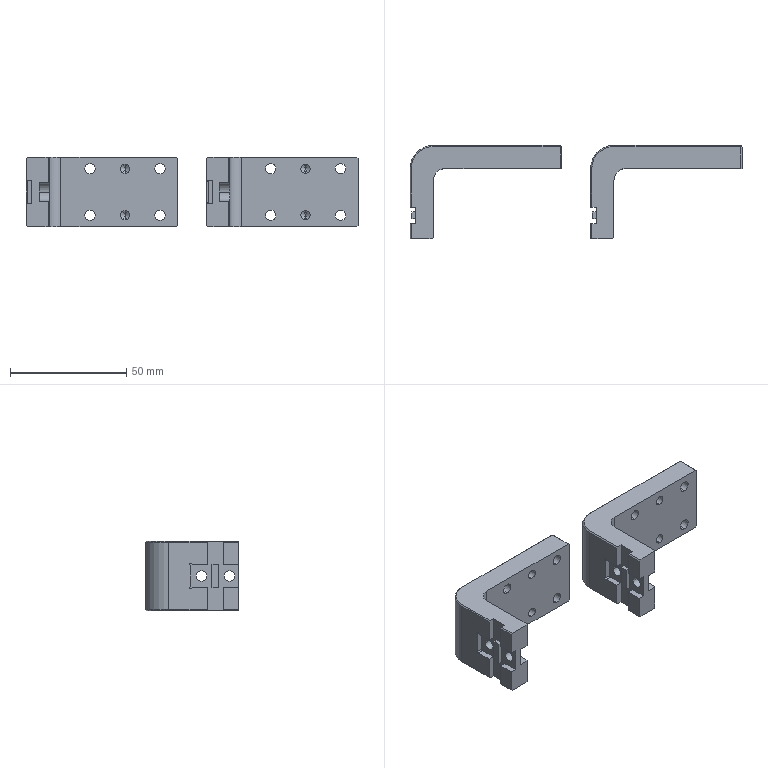NC program | NX | posted with a generic post | part box 142.5 x 40 x 30 mm
Whole program:
N10 G17 G21 G94 G90
(HOLE_MILLING , TOOL : D6)
N12 T12 M6
N14 G54
N16 G17 G0 G90 X-63.75 Y-5. B0. C0. S9500 M3
N18 G43 Z30. H12
N20 Z0.5
N22 G94 G3 X-64.25 Y-4.5 R0.5 F1500.
N24 X-64.75 Y-5. R0.5
N26 X-64.75 Y-5. Z0. I1. J0.
N28 X-64.75 Y-5. Z-0.5 I1. J0.
N30 X-64.75 Y-5. Z-1. I1. J0.
N32 X-64.75 Y-5. Z-1.5 I1. J0.
N34 X-64.75 Y-5. Z-2. I1. J0.
N36 X-64.75 Y-5. Z-2.5 I1. J0.
N38 X-64.75 Y-5. Z-3. I1. J0.
N40 X-64.75 Y-5. Z-3.5 I1. J0.
N42 X-64.75 Y-5. Z-4. I1. J0.
N44 X-64.75 Y-5. Z-4.5 I1. J0.
N46 X-64.059 Y-5.951 Z-4.6 R1.
N48 X-62.799 Y-5.309 R1.
N50 X-64.059 Y-5.951 R-1.
N52 X-63.429 Y-5.63 R0.5
N54 X-63.75 Y-5. R0.5
N56 G0 Z30.
N58 Y-25.
N60 Z0.5
N62 G3 X-64.25 Y-24.5 R0.5
N64 X-64.75 Y-25. R0.5
N66 X-64.75 Y-25. Z0. I1. J0.
N68 X-64.75 Y-25. Z-0.5 I1. J0.
N70 X-64.75 Y-25. Z-1. I1. J0.
N72 X-64.75 Y-25. Z-1.5 I1. J0.
N74 X-64.75 Y-25. Z-2. I1. J0.
N76 X-64.75 Y-25. Z-2.5 I1. J0.
N78 X-64.75 Y-25. Z-3. I1. J0.
N80 X-64.75 Y-25. Z-3.5 I1. J0.
N82 X-64.75 Y-25. Z-4. I1. J0.
N84 X-64.75 Y-25. Z-4.5 I1. J0.
N86 X-64.059 Y-25.951 Z-4.6 R1.
N88 X-62.799 Y-25.309 R1.
N90 X-64.059 Y-25.951 R-1.
N92 X-63.429 Y-25.63 R0.5
N94 X-63.75 Y-25. R0.5
N96 G0 Z30.
N98 X-33.75
N100 Z0.5
N102 G3 X-34.25 Y-24.5 R0.5
N104 X-34.75 Y-25. R0.5
N106 X-34.75 Y-25. Z0. I1. J0.
N108 X-34.75 Y-25. Z-0.5 I1. J0.
N110 X-34.75 Y-25. Z-1. I1. J0.
N112 X-34.75 Y-25. Z-1.5 I1. J0.
N114 X-34.75 Y-25. Z-2. I1. J0.
N116 X-34.75 Y-25. Z-2.5 I1. J0.
N118 X-34.75 Y-25. Z-3. I1. J0.
N120 X-34.75 Y-25. Z-3.5 I1. J0.
N122 X-34.75 Y-25. Z-4. I1. J0.
N124 X-34.75 Y-25. Z-4.5 I1. J0.
N126 X-34.059 Y-25.951 Z-4.6 R1.
N128 X-32.799 Y-25.309 R1.
N130 X-34.059 Y-25.951 R-1.
N132 X-33.429 Y-25.63 R0.5
N134 X-33.75 Y-25. R0.5
N136 G0 Z30.
N138 Y-5.
N140 Z0.5
N142 G3 X-34.25 Y-4.5 R0.5
N144 X-34.75 Y-5. R0.5
N146 X-34.75 Y-5. Z0. I1. J0.
N148 X-34.75 Y-5. Z-0.5 I1. J0.
N150 X-34.75 Y-5. Z-1. I1. J0.
N152 X-34.75 Y-5. Z-1.5 I1. J0.
N154 X-34.75 Y-5. Z-2. I1. J0.
N156 X-34.75 Y-5. Z-2.5 I1. J0.
N158 X-34.75 Y-5. Z-3. I1. J0.
N160 X-34.75 Y-5. Z-3.5 I1. J0.
N162 X-34.75 Y-5. Z-4. I1. J0.
N164 X-34.75 Y-5. Z-4.5 I1. J0.
N166 X-34.059 Y-5.951 Z-4.6 R1.
N168 X-32.799 Y-5.309 R1.
N170 X-34.059 Y-5.951 R-1.
N172 X-33.429 Y-5.63 R0.5
N174 X-33.75 Y-5. R0.5
N176 G0 Z30.
N178 X13.75
N180 Z0.5
N182 G3 X13.25 Y-4.5 R0.5
N184 X12.75 Y-5. R0.5
N186 X12.75 Y-5. Z0. I1. J0.
N188 X12.75 Y-5. Z-0.5 I1. J0.
N190 X12.75 Y-5. Z-1. I1. J0.
N192 X12.75 Y-5. Z-1.5 I1. J0.
N194 X12.75 Y-5. Z-2. I1. J0.
N196 X12.75 Y-5. Z-2.5 I1. J0.
N198 X12.75 Y-5. Z-3. I1. J0.
N200 X12.75 Y-5. Z-3.5 I1. J0.
N202 X12.75 Y-5. Z-4. I1. J0.
N204 X12.75 Y-5. Z-4.5 I1. J0.
N206 X13.441 Y-5.951 Z-4.6 R1.
N208 X14.701 Y-5.309 R1.
N210 X13.441 Y-5.951 R-1.
N212 X14.071 Y-5.63 R0.5
N214 X13.75 Y-5. R0.5
N216 G0 Z30.
N218 Y-25.
N220 Z0.5
N222 G3 X13.25 Y-24.5 R0.5
N224 X12.75 Y-25. R0.5
N226 X12.75 Y-25. Z0. I1. J0.
N228 X12.75 Y-25. Z-0.5 I1. J0.
N230 X12.75 Y-25. Z-1. I1. J0.
N232 X12.75 Y-25. Z-1.5 I1. J0.
N234 X12.75 Y-25. Z-2. I1. J0.
N236 X12.75 Y-25. Z-2.5 I1. J0.
N238 X12.75 Y-25. Z-3. I1. J0.
N240 X12.75 Y-25. Z-3.5 I1. J0.
N242 X12.75 Y-25. Z-4. I1. J0.
N244 X12.75 Y-25. Z-4.5 I1. J0.
N246 X13.441 Y-25.951 Z-4.6 R1.
N248 X14.701 Y-25.309 R1.
N250 X13.441 Y-25.951 R-1.
N252 X14.071 Y-25.63 R0.5
N254 X13.75 Y-25. R0.5
N256 G0 Z30.
N258 X43.75
N260 Z0.5
N262 G3 X43.25 Y-24.5 R0.5
N264 X42.75 Y-25. R0.5
N266 X42.75 Y-25. Z0. I1. J0.
N268 X42.75 Y-25. Z-0.5 I1. J0.
N270 X42.75 Y-25. Z-1. I1. J0.
N272 X42.75 Y-25. Z-1.5 I1. J0.
N274 X42.75 Y-25. Z-2. I1. J0.
N276 X42.75 Y-25. Z-2.5 I1. J0.
N278 X42.75 Y-25. Z-3. I1. J0.
N280 X42.75 Y-25. Z-3.5 I1. J0.
N282 X42.75 Y-25. Z-4. I1. J0.
N284 X42.75 Y-25. Z-4.5 I1. J0.
N286 X43.441 Y-25.951 Z-4.6 R1.
N288 X44.701 Y-25.309 R1.
N290 X43.441 Y-25.951 R-1.
N292 X44.071 Y-25.63 R0.5
N294 X43.75 Y-25. R0.5
N296 G0 Z30.
N298 Y-5.
N300 Z0.5
N302 G3 X43.25 Y-4.5 R0.5
N304 X42.75 Y-5. R0.5
N306 X42.75 Y-5. Z0. I1. J0.
N308 X42.75 Y-5. Z-0.5 I1. J0.
N310 X42.75 Y-5. Z-1. I1. J0.
N312 X42.75 Y-5. Z-1.5 I1. J0.
N314 X42.75 Y-5. Z-2. I1. J0.
N316 X42.75 Y-5. Z-2.5 I1. J0.
N318 X42.75 Y-5. Z-3. I1. J0.
N320 X42.75 Y-5. Z-3.5 I1. J0.
N322 X42.75 Y-5. Z-4. I1. J0.
N324 X42.75 Y-5. Z-4.5 I1. J0.
N326 X43.441 Y-5.951 Z-4.6 R1.
N328 X44.701 Y-5.309 R1.
N330 X43.441 Y-5.951 R-1.
N332 X44.071 Y-5.63 R0.5
N334 X43.75 Y-5. R0.5
N336 G0 Z30.
N338 M5
N340 M2